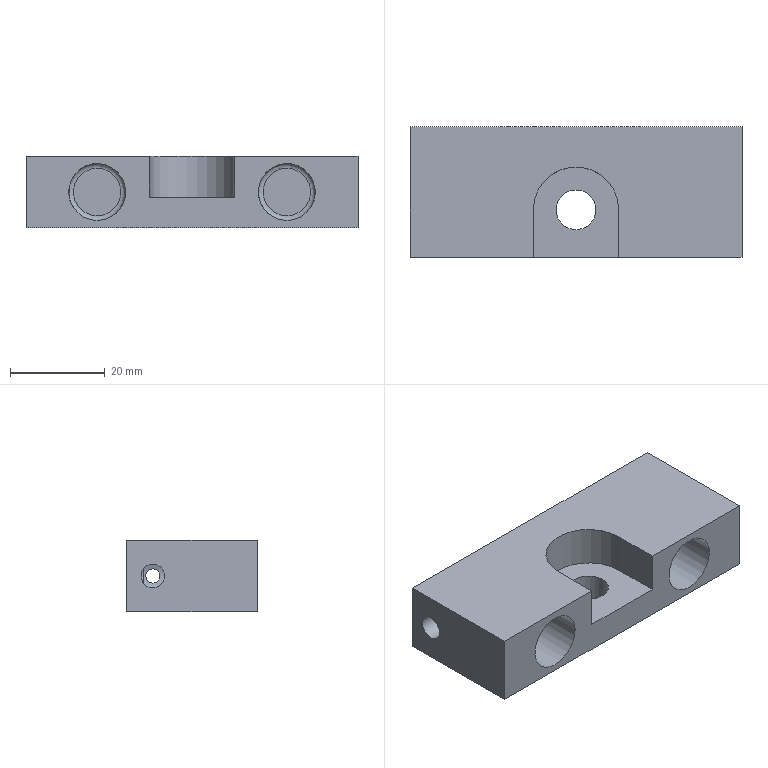NC program | NX | posted with a generic post | part box 70 x 27.5 x 15 mm
Lines 1 to 1563 of 3352, first 1339 of 1557 lines:
N10 G17 G21 G94 G90
(PLANAR_MILL_COPY , TOOL : D50面刀)
N12 T01 M6
N14 G53
N16 G17 G0 G90 X-0.05 Y-65. B0. C0. S1600 M3
N18 G43 Z20. H1
N20 Z3.05
N22 G94 G1 Z0.05 F800.
N24 Y-35.
N26 Y35.
N28 Y65.
N30 Z3.05
N32 G0 Z20.
N34 M5
(ADAPTIVE_MILLING , TOOL : D10-30-D10-75-3T-ROUGH)
N36 T02 M6
N38 G53
N40 G17 G0 G90 X-0.54 Y47.029 B0. C0. S3000 M3
N42 G43 Z20. H2
N44 Z-13.
N46 G94 G1 X-0.546 Y46.879 Z-13.937 F1500.
N48 X-0.553 Y46.729 Z-14.308
N50 X-0.559 Y46.579 Z-14.58
N52 X-0.566 Y46.43 Z-14.8
N54 X-0.572 Y46.28 Z-14.984
N56 X-0.579 Y46.13 Z-15.142
N58 X-0.586 Y45.98 Z-15.28
N60 X-0.592 Y45.83 Z-15.4
N62 X-0.599 Y45.68 Z-15.505
N64 X-0.605 Y45.53 Z-15.598
N66 X-0.612 Y45.381 Z-15.679
N68 X-0.618 Y45.231 Z-15.75
N70 X-0.625 Y45.081 Z-15.81
N72 X-0.631 Y44.931 Z-15.862
N74 X-0.638 Y44.781 Z-15.905
N76 X-0.644 Y44.631 Z-15.939
N78 X-0.651 Y44.481 Z-15.966
N80 X-0.657 Y44.332 Z-15.985
N82 X-0.664 Y44.182 Z-15.996
N84 X-0.67 Y44.032 Z-16.
N86 X-0.736 Y42.523
N88 G3 X0.007 Y41.505 R1.01
N90 X2.762 Y41.25 R14.191
N92 X13.643 Y41.189 R765.773
N94 G2 X17.871 Y38.648 R5.724
N96 X19.406 Y34.419 R9.683
N98 X19.682 Y29.331 R40.052
N100 G1 X19.699 Y22.431
N102 X19.698 Y-34.945
N104 G2 X17.285 Y-39.28 R5.638
N106 X12.977 Y-40.9 R9.483
N108 X7.401 Y-41.187 R42.459
N110 G1 X1.251 Y-41.2
N112 X-13.457 Y-41.198
N114 G2 X-17.775 Y-38.771 R5.666
N116 X-19.389 Y-34.525 R9.459
N118 X-19.681 Y-29.4 R38.334
N120 G1 X-19.699 Y-22.425
N122 X-19.697 Y34.946
N124 G2 X-17.282 Y39.268 R5.662
N126 X-13.075 Y40.881 R9.398
N128 X-7.988 Y41.181 R37.246
N130 X-1.014 Y41.164 R160.579
N132 G3 X9.001 Y40.903 R137.343
N134 G2 X12.406 Y40.86 R48.622
N136 X15.192 Y39.92 R6.998
N138 G1 X15.722 Y39.757
N140 G2 X17.393 Y38.64 R5.993
N142 X18.508 Y36.969 R5.993
N144 X19.081 Y34.188 R11.725
N146 X19.383 Y27.636 R61.147
N148 G1 X19.399 Y20.661
N150 X19.398 Y-33.278
N152 G2 X18.8 Y-36.008 R7.984
N154 X18.031 Y-37.862 R6.016
N156 X16.61 Y-39.283 R5.993
N158 X14.177 Y-40.223 R7.334
N160 X8.446 Y-40.842 R28.015
N162 X0.271 Y-40.899 R504.458
N164 G1 X-12.054 Y-40.887
N166 G2 X-15.177 Y-39.924 R6.927
N168 G1 X-15.722 Y-39.757
N170 G2 X-17.393 Y-38.64 R5.993
N172 X-18.508 Y-36.969 R5.993
N174 X-19.089 Y-34.118 R11.94
N176 X-19.388 Y-26.965 R67.131
N178 G1 X-19.399 Y-20.59
N180 X-19.398 Y33.255
N182 G2 X-18.803 Y35.985 R7.776
N184 X-18.031 Y37.862 R5.939
N186 X-16.61 Y39.283 R5.993
N188 X-14.212 Y40.213 R7.235
N190 X-8.557 Y40.838 R27.584
N192 X-3.607 Y40.895 R550.386
N194 X9.582 Y40.88 R989.035
N196 G3 X11.662 Y40.601 R75.414
N198 G2 X13.481 Y40.154 R43.193
N200 X15.722 Y39.757 R6.086
N202 X17.393 Y38.64 R5.993
N204 X18.508 Y36.969 R5.993
N206 X18.9 Y34.999 R5.998
N208 G3 X19.057 Y29. R461.095
N210 G2 X19.099 Y19.4 R690.026
N212 G1 X19.093 Y-32.197
N214 G2 X18.9 Y-33.872 R19.687
N216 X18.801 Y-36.006 R11.828
N218 G1 X18.735 Y-36.221
N220 G3 X20.129 Y-37.412 R1.
N222 X20.586 Y-36.97 Z-15.968 R1.088
N224 G1 X21.31 Y-35.839 Z-15.9
N226 X21.969 Y-34.809 F15000.
N228 G3 X22.127 Y-34.263 R1.011
N230 G1 X21.669 Y31.517
N232 X21.658 Y31.648
N234 X21.633 Y31.777
N236 X21.391 Y32.652
N238 X20.859 Y34.569 Z-16. F1500.
N240 G3 X18.9 Y34.287 R1.
N242 G1 Y-35.001
N244 G2 X18.507 Y-36.972 R5.996
N246 X17.39 Y-38.643 R5.993
N248 X15.719 Y-39.758 R5.993
N250 X13.749 Y-40.15 R5.998
N252 X4.104 Y-40.588 R90.538
N254 G1 X-2.421 Y-40.599
N256 G2 X-10.891 Y-40.577 R486.467
N258 X-13.286 Y-40.152 R14.802
N260 X-14.756 Y-40.051 R10.569
N262 G1 X-15.223 Y-39.909
N264 G3 X-16.353 Y-41.41 R1.
N266 X-15.967 Y-41.762 Z-15.974 R1.15
N268 G1 X-14.733 Y-42.546 Z-15.9
N270 X-13.791 Y-43.145 F15000.
N272 G3 X-13.264 Y-43.301 R1.013
N274 G1 X11.791 Y-43.542
N276 G3 X12.382 Y-43.356 R1.009
N278 G1 X13.375 Y-42.646
N280 X14.383 Y-41.921 Z-15.963 F1500.
N282 G3 X14.74 Y-41.285 Z-16. R1.001
N284 X13.749 Y-40.15 R1.
N286 X6.074 Y-40.264 R279.217
N288 G2 X-9.795 Y-40.283 R887.959
N290 G1 X-11.175 Y-40.15
N292 X-13.35
N294 G3 X-13.663 Y-42.1 R1.
N296 G1 X-11.746 Y-42.633 Z-15.9
N298 X-11.233 Y-42.78 F15000.
N300 X-10.716 Y-42.91
N302 X-10.581 Y-42.919
N304 X8.467
N306 X8.602 Y-42.908
N308 X8.735 Y-42.883
N310 X9.608 Y-42.64
N312 X11.525 Y-42.108 Z-16. F1500.
N314 G3 X11.237 Y-40.15 R1.
N316 G1 X-13.751
N318 G2 X-15.722 Y-39.757 R5.996
N320 X-17.393 Y-38.64 R5.993
N322 X-18.508 Y-36.969 R5.993
N324 X-18.9 Y-34.999 R5.998
N326 G3 X-19.058 Y-28.948 R473.561
N328 G2 X-19.099 Y-19.424 R689.078
N330 G1 X-19.097 Y31.83
N332 G2 X-18.9 Y33.843 R14.392
N334 X-18.801 Y36.006 R11.963
N336 G3 X-20.035 Y37.075 R1.
N338 X-20.677 Y36.588 Z-15.958 R1.059
N340 G1 X-21.331 Y35.628 Z-15.9
N342 X-22.019 Y34.619 F15000.
N344 G3 X-22.193 Y34.048 R1.009
N346 G1 X-21.669 Y-31.517
N348 X-21.658 Y-31.648
N350 X-21.633 Y-31.776
N352 X-21.391 Y-32.651
N354 X-20.859 Y-34.569 Z-16. F1500.
N356 G3 X-18.9 Y-34.287 R1.
N358 G1 Y35.001
N360 G2 X-18.507 Y36.972 R5.996
N362 X-17.39 Y38.643 R5.993
N364 X-15.719 Y39.758 R5.993
N366 X-13.75 Y40.15 R5.999
N368 X-3.9 Y40.588 R91.992
N370 G1 X1.425 Y40.595
N372 X8.533 Y40.593
N374 G2 X11.957 Y40.15 R25.662
N376 G1 X13.532
N378 G3 X14.526 Y41.262 R1.
N380 X14.033 Y42.02 Z-15.953 R1.045
N382 G1 X13.175 Y42.631 Z-15.9
N384 X12.153 Y43.357 F15000.
N386 G3 X11.574 Y43.542 R1.008
N388 G1 X-11.792
N390 G3 X-12.371 Y43.357 R1.008
N392 G1 X-13.372 Y42.646
N394 X-14.382 Y41.922 Z-15.963 F1500.
N396 G3 X-14.74 Y41.288 Z-16. R1.001
N398 X-13.75 Y40.15 R1.
N400 X-6.022 Y40.264 R288.131
N402 G2 X7.82 Y40.273 R666.629
N404 G1 X9.517 Y40.15
N406 X11.992
N408 G3 X12.305 Y42.1 R1.
N410 G1 X10.388 Y42.633 Z-15.9
N412 X9.875 Y42.78 F15000.
N414 X9.358 Y42.91
N416 X9.223 Y42.919
N418 X-8.506
N420 X-8.64 Y42.908
N422 X-8.773 Y42.883
N424 X-9.646 Y42.64
N426 X-11.563 Y42.108 Z-16. F1500.
N428 G3 X-11.275 Y40.15 R1.
N430 G1 X9.537
N432 G3 X10.535 Y41.321 R1.01
N434 G1 X10.322 Y42.637
N436 X10.298 Y42.785 Z-15.996
N438 X10.274 Y42.933 Z-15.985
N440 X10.25 Y43.081 Z-15.966
N442 X10.227 Y43.229 Z-15.939
N444 X10.203 Y43.377 Z-15.905
N446 X10.179 Y43.525 Z-15.862
N448 X10.155 Y43.673 Z-15.81
N450 X10.131 Y43.821 Z-15.75
N452 X10.107 Y43.969 Z-15.679
N454 X10.083 Y44.118 Z-15.598
N456 X10.059 Y44.266 Z-15.505
N458 X10.035 Y44.414 Z-15.4
N460 X10.011 Y44.562 Z-15.28
N462 X9.988 Y44.71 Z-15.142
N464 X9.964 Y44.858 Z-14.984
N466 X9.94 Y45.006 Z-14.8
N468 X9.916 Y45.154 Z-14.58
N470 X9.892 Y45.302 Z-14.308
N472 X9.868 Y45.45 Z-13.937
N474 X9.844 Y45.598 Z-13.
N476 G0 Z20.
N478 X-24.359 Y-10.135
N480 Z-5.499
N482 G1 X-24.21 Y-10.115 Z-6.436
N484 X-24.062 Y-10.095 Z-6.807
N486 X-23.913 Y-10.074 Z-7.079
N488 X-23.765 Y-10.054 Z-7.299
N490 X-23.616 Y-10.034 Z-7.483
N492 X-23.467 Y-10.014 Z-7.641
N494 X-23.319 Y-9.993 Z-7.779
N496 X-23.17 Y-9.973 Z-7.899
N498 X-23.021 Y-9.953 Z-8.004
N500 X-22.873 Y-9.932 Z-8.097
N502 X-22.724 Y-9.912 Z-8.178
N504 X-22.576 Y-9.892 Z-8.249
N506 X-22.427 Y-9.871 Z-8.309
N508 X-22.278 Y-9.851 Z-8.361
N510 X-22.13 Y-9.831 Z-8.404
N512 X-21.981 Y-9.81 Z-8.438
N514 X-21.833 Y-9.79 Z-8.465
N516 X-21.684 Y-9.77 Z-8.484
N518 X-21.535 Y-9.749 Z-8.495
N520 X-21.387 Y-9.729 Z-8.499
N522 X-19.729 Y-9.503
N524 G3 X-18.861 Y-8.601 R1.01
N526 X-18.61 Y-3.113 R44.979
N528 X-18.604 Y7.322 R791.192
N530 G2 X-18.864 Y8.631 R4.427
N532 G3 X-21.014 Y8.833 R1.1
N534 X-21.057 Y8.32 Z-8.473 R1.658
N536 G1 X-21.047 Y6.847 Z-8.399
N538 X-20.961 Y-6.535 F15000.
N540 X-20.948 Y-7.751 Z-8.46 F1500.
N542 G3 X-20.641 Y-8.442 Z-8.499 R1.101
N544 X-18.801 Y-7.994 R1.1
N546 X-18.4 Y-5.172 R11.11
N548 X-18.323 Y6.524 R244.406
N550 G1 X-18.411 Y6.848
N552 G3 X-19.933 Y7.308 R1.1
N554 X-20.494 Y6.285 Z-8.437 R1.133
N556 G1 X-20.515 Y5.523 Z-8.399
N558 X-20.832 Y-6.142 F15000.
N560 X-20.862 Y-7.434 Z-8.464 F1500.
N562 G3 X-20.624 Y-8.075 Z-8.499 R1.102
N564 X-18.713 Y-7.707 R1.1
N566 X-18.124 Y-4.24 R12.163
N568 X-18.029 Y5.649 R169.285
N570 X-18.164 Y6.386 R2.632
N572 G2 X-18.628 Y7.425 R3.79
N574 G3 X-20.442 Y7.9 R1.1
N576 X-20.779 Y6.991 Z-8.449 R1.147
N578 G1 X-20.764 Y6.004 Z-8.399
N580 X-20.59 Y-5.636 F15000.
N582 X-20.57 Y-6.604 Z-8.448 F1500.
N584 G3 X-20.058 Y-7.444 Z-8.499 R1.099
N586 X-18.507 Y-7.028 R1.1
N588 X-17.96 Y-4.778 R6.799
N590 X-17.713 Y1.504 R64.517
N592 X-17.785 Y5.427 R37.651
N594 X-17.984 Y6.075 R1.569
N596 X-19.388 Y6.427 R1.1
N598 X-19.99 Y5.405 Z-8.436 R1.127
N600 G1 X-20.024 Y4.667 Z-8.399
N602 X-20.481 Y-5.436 F15000.
N604 X-20.521 Y-6.436 Z-8.449 F1500.
N606 G3 X-20.089 Y-7.286 Z-8.499 R1.099
N608 X-18.454 Y-6.929 R1.1
N610 X-17.731 Y-4.48 R6.474
N612 X-17.422 Y1.708 R53.159
N614 X-17.541 Y5.13 R22.267
N616 X-18.033 Y6.14 R1.665
N618 G1 X-18.174 Y6.405
N620 G3 X-19.711 Y6.829 R1.1
N622 X-20.245 Y5.8 Z-8.438 R1.133
N624 G1 X-20.252 Y5.03 Z-8.399
N626 X-20.34 Y-5.168 F15000.
N628 X-20.342 Y-6.147 Z-8.448 F1500.
N630 G3 X-19.86 Y-6.993 Z-8.499 R1.099
N632 X-18.277 Y-6.598 R1.1
N634 X-17.479 Y-4.048 R6.758
N636 X-17.198 Y4.121 R47.526
N638 X-17.535 Y5.528 R3.358
N640 G1 X-17.818 Y5.878
N642 G3 X-19.188 Y6.149 R1.1
N644 X-19.77 Y5.122 Z-8.437 R1.128
N646 G1 X-19.794 Y4.377 Z-8.399
N648 X-20.088 Y-4.732 F15000.
N650 X-20.114 Y-5.693 Z-8.447 F1500.
N652 G3 X-19.635 Y-6.559 Z-8.499 R1.099
N654 X-18.047 Y-6.168 R1.1
N656 X-17.31 Y-4.123 R5.453
N658 X-16.865 Y1.668 R34.498
N660 X-17.096 Y4.751 R13.069
N662 X-17.379 Y5.348 R1.45
N664 X-18.583 Y5.473 R1.101
N666 X-19.18 Y4.487 Z-8.438 R1.134
N668 G1 X-19.241 Y3.711 Z-8.399
N670 X-19.887 Y-4.47 F15000.
N672 X-19.954 Y-5.405 Z-8.446 F1500.
N674 G3 X-19.496 Y-6.306 Z-8.499 R1.099
N676 X-18.007 Y-6.109 R1.1
N678 X-17.173 Y-4.263 R4.393
N680 X-16.612 Y0.923 R25.278
N682 X-16.83 Y4.394 R14.374
N684 X-17.249 Y5.242 R1.676
N686 X-18.475 Y5.353 R1.1
N688 X-19.048 Y4.387 Z-8.44 R1.131
N690 G1 X-19.113 Y3.577 Z-8.399
N692 X-19.743 Y-4.295 F15000.
N694 X-19.812 Y-5.23 Z-8.446 F1500.
N696 G3 X-19.355 Y-6.131 Z-8.499 R1.099
N698 X-17.865 Y-5.935 R1.1
N700 X-16.918 Y-3.908 R4.707
N702 X-16.461 Y3.485 R23.099
N704 X-16.927 Y4.948 R3.387
N706 X-17.393 Y5.36 R12.87
N708 G1 X-17.559 Y5.563
N710 G3 X-18.947 Y5.825 R1.1
N712 X-19.511 Y4.785 Z-8.436 R1.128
N714 G1 X-19.519 Y4.042 Z-8.399
N716 X-19.614 Y-4.137 F15000.
N718 X-19.619 Y-5.073 Z-8.446 F1500.
N720 G3 X-19.101 Y-5.942 Z-8.499 R1.099
N722 X-17.674 Y-5.703 R1.1
N724 X-16.676 Y-3.628 R4.873
N726 X-16.221 Y3.267 R19.842
N728 X-16.713 Y4.773 R3.545
N730 G1 X-17.055 Y5.083
N732 G3 X-18.304 Y5.185 R1.1
N734 X-18.857 Y4.21 Z-8.44 R1.131
N736 G1 X-18.907 Y3.396 Z-8.399
N738 X-19.355 Y-3.822 F15000.
N740 X-19.407 Y-4.757 Z-8.446 F1500.
N742 G3 X-18.933 Y-5.651 Z-8.499 R1.099
N744 X-17.46 Y-5.442 R1.1
N746 X-16.448 Y-3.413 R4.805
N748 X-15.99 Y3.086 R17.275
N750 X-16.502 Y4.606 R3.475
N752 G1 X-16.605 Y4.714
N754 G3 X-17.695 Y4.721 R1.101
N756 X-18.259 Y3.791 Z-8.442 R1.135
N758 G1 X-18.355 Y2.943 Z-8.399
N760 X-19.085 Y-3.532 F15000.
N762 X-19.184 Y-4.464 Z-8.446 F1500.
N764 G3 X-18.757 Y-5.38 Z-8.499 R1.099
N766 X-17.39 Y-5.357 R1.1
N768 X-16.443 Y-3.867 R3.519
N770 X-15.796 Y3.107 R14.715
N772 X-16.339 Y4.508 R3.093
N774 G1 X-16.508 Y4.656
N776 G3 X-17.672 Y4.687 R1.076
N778 X-18.193 Y3.791 Z-8.445 R1.108
N780 G1 X-18.289 Y2.887 Z-8.399
N782 X-18.956 Y-3.418 F15000.
N784 X-19.057 Y-4.417 Z-8.45 F1500.
N786 G3 X-18.669 Y-5.284 Z-8.499 R1.074
N788 X-17.303 Y-5.286 R1.075
N790 X-16.245 Y-3.739 R3.537
N792 X-15.582 Y2.989 R13.284
N794 X-16.211 Y4.462 R2.96
N796 G1 X-16.389 Y4.6
N798 G3 X-17.497 Y4.558 R1.101
N800 X-18.011 Y3.665 Z-8.445 R1.135
N802 G1 X-18.116 Y2.752 Z-8.399
N804 X-18.82 Y-3.305 F15000.
N806 X-18.923 Y-4.246 Z-8.447 F1500.
N808 G3 X-18.506 Y-5.158 Z-8.499 R1.099
N810 X-17.13 Y-5.143 R1.1
N812 X-15.966 Y-3.424 R3.809
N814 X-15.372 Y2.873 R12.173
N816 X-16.029 Y4.366 R3.073
N818 X-16.612 Y4.719 R3.315
N820 G1 X-16.844 Y4.909
N822 G3 X-18.123 Y4.993 R1.1
N824 X-18.643 Y3.972 Z-8.439 R1.135
N826 G1 X-18.651 Y3.186 Z-8.399
N828 X-18.715 Y-3.217 F15000.
N830 X-18.719 Y-4.193 Z-8.448 F1500.
N832 G3 X-18.235 Y-5.041 Z-8.499 R1.099
N834 X-16.927 Y-4.977 R1.1
N836 X-15.766 Y-3.309 R3.83
N838 X-15.188 Y2.856 R11.082
N840 X-15.852 Y4.278 R2.951
N842 G1 X-16.213 Y4.505
N844 G3 X-17.353 Y4.443 R1.101
N846 X-17.836 Y3.543 Z-8.446 R1.141
N848 G1 X-17.921 Y2.618 Z-8.399
N850 X-18.437 Y-2.99 F15000.
N852 X-18.518 Y-3.939 Z-8.447 F1500.
N854 G3 X-18.084 Y-4.838 Z-8.499 R1.099
N856 X-16.724 Y-4.81 R1.1
N858 X-15.513 Y-3.07 R3.925
N860 X-14.989 Y2.763 R10.298
N862 X-15.669 Y4.184 R2.932
N864 G1 X-16.019 Y4.401
N866 G3 X-17.169 Y4.332 R1.101
N868 X-17.641 Y3.429 Z-8.446 R1.141
N870 G1 X-17.718 Y2.5 Z-8.399
N872 X-18.151 Y-2.758 F15000.
N874 X-18.225 Y-3.734 Z-8.448 F1500.
N876 G3 X-17.806 Y-4.613 Z-8.499 R1.099
N878 X-16.61 Y-4.717 R1.101
N880 X-15.502 Y-3.375 R3.126
N882 X-14.824 Y2.793 R9.464
N884 X-15.501 Y4.105 R2.672
N886 G1 X-15.689 Y4.229
N888 G3 X-16.713 Y4.111 R1.101
N890 X-17.192 Y3.261 Z-8.448 R1.146
N892 G1 X-17.329 Y2.29 Z-8.399
N894 X-18.026 Y-2.669 F15000.
N896 X-18.157 Y-3.636 Z-8.448 F1500.
N898 G3 X-17.786 Y-4.54 Z-8.499 R1.099
N900 X-16.544 Y-4.682 R1.1
N902 X-15.34 Y-3.336 R3.03
N904 X-14.661 Y2.809 R8.843
N906 X-15.389 Y4.082 R2.488
N908 G1 X-15.584 Y4.194
N910 G3 X-16.642 Y4.071 R1.076
N912 X-17.083 Y3.254 Z-8.451 R1.12
N914 G1 X-17.219 Y2.231 Z-8.399
N916 X-17.856 Y-2.561 F15000.
N918 X-17.988 Y-3.594 Z-8.451 F1500.
N920 G3 X-17.653 Y-4.447 Z-8.499 R1.075
N922 X-16.411 Y-4.611 R1.075
N924 X-15.16 Y-3.267 R3.047
N926 X-14.482 Y2.764 R8.386
N928 X-15.255 Y4.05 R2.497
N930 G1 X-15.487 Y4.171
N932 G3 X-16.479 Y3.989 R1.101
N934 X-16.909 Y3.181 Z-8.452 R1.147
N936 G1 X-17.058 Y2.144 Z-8.399
N938 X-17.722 Y-2.486 F15000.
N940 X-17.859 Y-3.472 Z-8.449 F1500.
N942 G3 X-17.507 Y-4.364 Z-8.499 R1.099
N944 X-16.246 Y-4.523 R1.1
N946 X-14.951 Y-3.148 R3.109
N948 X-14.321 Y2.761 R7.947
N950 X-15.123 Y4.021 R2.428
N952 X-15.722 Y4.243 R2.988
N954 G1 X-15.821 Y4.296
N956 G3 X-16.992 Y4.212 R1.101
N958 X-17.443 Y3.272 Z-8.445 R1.134
N960 G1 X-17.473 Y2.367 Z-8.399
N962 X-17.633 Y-2.437 F15000.
N964 X-17.655 Y-2.996 Z-8.427 F1500.
N966 X-17.66 Y-3.555 Z-8.455
N968 G3 X-17.258 Y-4.301 Z-8.499 R1.116
N970 X-16.048 Y-4.417 R1.101
N972 X-14.743 Y-3.032 R3.144
N974 X-14.136 Y2.681 R7.63
N976 X-14.939 Y3.959 R2.556
N978 X-15.352 Y4.13 R2.709
N980 X-16.379 Y3.92 R1.101
N982 X-16.776 Y3.101 Z-8.452 R1.148
N984 G1 X-16.889 Y2.054 Z-8.399
N986 X-17.36 Y-2.292 F15000.
N988 X-17.464 Y-3.297 Z-8.45 F1500.
N990 G3 X-17.093 Y-4.167 Z-8.499 R1.099
N992 X-15.849 Y-4.311 R1.1
N994 X-14.497 Y-2.846 R3.242
N996 X-13.955 Y2.608 R7.351
N998 X-14.786 Y3.919 R2.545
N1000 X-15.205 Y4.086 R3.378
N1002 X-16.259 Y3.853 R1.101
N1004 X-16.629 Y3.027 Z-8.452 R1.149
N1006 G1 X-16.716 Y1.973 Z-8.399
N1008 X-17.051 Y-2.127 F15000.
N1010 X-17.101 Y-2.684 Z-8.427 F1500.
N1012 X-17.133 Y-3.243 Z-8.455
N1014 G3 X-16.768 Y-4.008 Z-8.499 R1.116
N1016 X-15.719 Y-4.242 R1.101
N1018 X-14.47 Y-3.047 R2.783
N1020 X-13.824 Y2.677 R6.992
N1022 X-14.655 Y3.889 R2.357
N1024 G1 X-15.004 Y4.025
N1026 G3 X-16.061 Y3.788 R1.101
N1028 X-16.427 Y3.007 Z-8.455 R1.156
N1030 G1 X-16.554 Y1.909 Z-8.399
N1032 X-17.021 Y-2.111 F15000.
N1034 X-17.135 Y-3.136 Z-8.451 F1500.
N1036 G3 X-16.787 Y-3.995 Z-8.499 R1.1
N1038 X-15.719 Y-4.242 R1.101
N1040 X-14.423 Y-3.181 R2.503
N1042 X-13.661 Y2.65 R6.743
N1044 X-14.495 Y3.844 R2.327
N1046 G1 X-14.735 Y3.947
N1048 G3 X-15.624 Y3.661 R1.102
N1050 X-15.976 Y2.944 Z-8.458 R1.166
N1052 G1 X-16.172 Y1.787 Z-8.399
N1054 X-16.817 Y-2.007 F15000.
N1056 X-16.914 Y-2.555 Z-8.427 F1500.
N1058 X-16.994 Y-3.106 Z-8.455
N1060 G3 X-16.692 Y-3.904 Z-8.499 R1.116
N1062 X-15.576 Y-4.198 R1.101
N1064 X-14.281 Y-3.171 R2.53
N1066 X-13.506 Y2.644 R6.533
N1068 X-14.39 Y3.839 R2.261
N1070 G1 X-14.672 Y3.938
N1072 G3 X-15.612 Y3.656 R1.101
N1074 X-15.961 Y2.922 Z-8.457 R1.163
N1076 G1 X-16.133 Y1.776 Z-8.399
N1078 X-16.691 Y-1.947 F15000.
N1080 X-16.779 Y-2.512 Z-8.428 F1500.
N1082 X-16.851 Y-3.079 Z-8.457
N1084 G3 X-16.558 Y-3.85 Z-8.499 R1.116
N1086 X-15.432 Y-4.155 R1.101
N1088 X-14.034 Y-3.015 R2.664
N1090 X-13.354 Y2.637 R6.36
N1092 X-14.286 Y3.841 R2.249
N1094 G1 X-14.571 Y3.931
N1096 G3 X-15.474 Y3.618 R1.102
N1098 X-15.8 Y2.908 Z-8.459 R1.169
N1100 G1 X-15.982 Y1.73 Z-8.399
N1102 X-16.541 Y-1.891 F15000.
N1104 X-16.632 Y-2.459 Z-8.428 F1500.
N1106 X-16.707 Y-3.03 Z-8.457
N1108 G3 X-16.423 Y-3.797 Z-8.499 R1.116
N1110 X-15.289 Y-4.111 R1.101
N1112 X-13.932 Y-3.065 R2.58
N1114 X-13.237 Y2.709 R6.146
N1116 X-14.198 Y3.849 R2.143
N1118 G1 X-14.45 Y3.919
N1120 G3 X-15.352 Y3.583 R1.102
N1122 X-15.657 Y2.894 Z-8.46 R1.167
N1124 G1 X-15.838 Y1.686 Z-8.399
N1126 X-16.365 Y-1.833 F15000.
N1128 X-16.448 Y-2.376 Z-8.427 F1500.
N1130 X-16.522 Y-2.922 Z-8.454
N1132 G3 X-16.246 Y-3.74 Z-8.499 R1.1
N1134 X-15.109 Y-4.057 R1.101
N1136 X-13.748 Y-3. R2.604
N1138 X-13.048 Y2.612 R6.046
N1140 X-14.008 Y3.815 R2.338
N1142 X-14.756 Y3.949 R2.163
N1144 G1 X-14.828 Y3.971
N1146 G3 X-15.908 Y3.713 R1.101
N1148 X-16.249 Y2.844 Z-8.451 R1.145
N1150 G1 X-16.267 Y1.817 Z-8.399
N1152 X-16.33 Y-1.82 F15000.
N1154 X-16.345 Y-3.004 Z-8.459 F1500.
N1156 G3 X-16.03 Y-3.724 Z-8.499 R1.101
N1158 X-14.93 Y-4.002 R1.101
N1160 X-13.518 Y-2.871 R2.703
N1162 X-12.893 Y2.593 R5.932
N1164 X-13.881 Y3.808 R2.347
N1166 X-14.318 Y3.906 R2.088
N1168 X-15.244 Y3.547 R1.101
N1170 X-15.529 Y2.848 Z-8.46 R1.167
N1172 G1 X-15.673 Y1.636 Z-8.399
N1174 X-16.075 Y-1.744 F15000.
N1176 X-16.201 Y-2.855 Z-8.455 F1500.
N1178 G3 X-15.914 Y-3.652 Z-8.499 R1.1
N1180 X-14.786 Y-3.959 R1.101
N1182 X-13.383 Y-2.874 R2.623
N1184 X-12.784 Y2.674 R5.779
N1186 X-13.779 Y3.812 R2.199
N1188 X-14.203 Y3.895 R3.262
N1190 X-15.148 Y3.514 R1.101
N1192 X-15.415 Y2.813 Z-8.461 R1.168
N1194 G1 X-15.534 Y1.594 Z-8.399
N1196 X-15.852 Y-1.676 F15000.
N1198 X-15.958 Y-2.824 Z-8.457 F1500.
N1200 G3 X-15.678 Y-3.59 Z-8.499 R1.1
N1202 X-14.753 Y-3.949 R1.101
N1204 X-13.404 Y-3.074 R2.272
N1206 X-12.633 Y2.66 R5.667
N1208 X-13.608 Y3.788 R2.263
N1210 X-14.047 Y3.879 R2.429
N1212 X-15.006 Y3.482 R1.101
N1214 X-15.259 Y2.817 Z-8.463 R1.186
N1216 G1 X-15.408 Y1.559 Z-8.399
N1218 X-15.79 Y-1.658 F15000.
N1220 X-15.92 Y-2.797 Z-8.457 F1500.
N1222 G3 X-15.653 Y-3.574 Z-8.499 R1.1
N1224 X-14.716 Y-3.945 R1.101
N1226 X-13.364 Y-3.178 R2.142
N1228 X-12.529 Y2.743 R5.535
N1230 X-13.503 Y3.791 R2.11
N1232 G1 X-13.72 Y3.848
N1234 G3 X-14.661 Y3.418 R1.101
N1236 X-14.889 Y2.827 Z-8.467 R1.199
N1238 G1 X-15.1 Y1.495 Z-8.399
N1240 X-15.592 Y-1.599 F15000.
N1242 X-15.767 Y-2.739 Z-8.457 F1500.
N1244 G3 X-15.536 Y-3.52 Z-8.499 R1.1
N1246 X-14.567 Y-3.93 R1.101
N1248 X-13.136 Y-3.076 R2.291
N1250 X-12.38 Y2.732 R5.48
N1252 X-13.384 Y3.79 R2.106
N1254 G1 X-13.677 Y3.85
N1256 G3 X-14.559 Y3.404 R1.101
N1258 X-14.776 Y2.827 Z-8.468 R1.204
N1260 G1 X-14.991 Y1.479 Z-8.399
N1262 X-15.476 Y-1.564 F15000.
N1264 X-15.655 Y-2.725 Z-8.458 F1500.
N1266 G3 X-15.438 Y-3.49 Z-8.499 R1.101
N1268 X-14.455 Y-3.919 R1.101
N1270 X-13.09 Y-3.171 R2.202
N1272 X-12.232 Y2.723 R5.4
N1274 X-13.267 Y3.796 R2.115
N1276 X-13.863 Y3.861 R2.988
N1278 X-14.839 Y3.441 R1.101
N1280 X-15.075 Y2.757 Z-8.462 R1.183
N1282 G1 X-15.174 Y1.508 Z-8.399
N1284 X-15.416 Y-1.547 F15000.
N1286 X-15.469 Y-2.175 Z-8.431 F1500.
N1288 X-15.51 Y-2.804 Z-8.462
N1290 G3 X-15.284 Y-3.482 Z-8.499 R1.101
N1292 X-14.305 Y-3.905 R1.101
N1294 X-12.88 Y-3.095 R2.306
N1296 X-12.113 Y2.769 R5.347
N1298 X-13.153 Y3.801 R2.088
N1300 X-13.563 Y3.85 R2.846
N1302 X-14.452 Y3.397 R1.101
N1304 X-14.666 Y2.8 Z-8.467 R1.198
N1306 G1 X-14.844 Y1.465 Z-8.399
N1308 X-15.239 Y-1.505 F15000.
N1310 X-15.396 Y-2.723 Z-8.461 F1500.
N1312 G3 X-15.195 Y-3.44 Z-8.499 R1.102
N1314 X-14.193 Y-3.894 R1.101
N1316 X-12.727 Y-3.078 R2.302
N1318 X-11.966 Y2.761 R5.301
N1320 X-13.01 Y3.799 R2.138
N1322 X-13.435 Y3.85 R2.424
N1324 X-14.331 Y3.387 R1.101
N1326 X-14.538 Y2.795 Z-8.467 R1.201
N1328 G1 X-14.712 Y1.452 Z-8.399
N1330 X-15.092 Y-1.483 F15000.
N1332 X-15.247 Y-2.711 Z-8.461 F1500.
N1334 G3 X-15.05 Y-3.42 Z-8.499 R1.102
N1336 X-14.044 Y-3.879 R1.101
N1338 X-12.575 Y-3.063 R2.313
N1340 X-11.819 Y2.754 R5.263
N1342 X-12.881 Y3.802 R2.143
N1344 X-13.288 Y3.85 R2.966
N1346 X-14.193 Y3.375 R1.101
N1348 X-14.392 Y2.794 Z-8.468 R1.205
N1350 G1 X-14.567 Y1.437 Z-8.399
N1352 X-14.943 Y-1.463 F15000.
N1354 X-15.031 Y-2.113 Z-8.432 F1500.
N1356 X-15.103 Y-2.764 Z-8.465
N1358 G3 X-14.903 Y-3.401 Z-8.499 R1.129
N1360 X-13.895 Y-3.864 R1.101
N1362 X-12.348 Y-2.967 R2.398
N1364 X-11.683 Y2.766 R5.23
N1366 X-12.77 Y3.81 R2.108
N1368 X-13.158 Y3.85 R5.359
N1370 X-14.07 Y3.365 R1.101
N1372 X-14.262 Y2.771 Z-8.467 R1.201
N1374 G1 X-14.407 Y1.422 Z-8.399
N1376 X-14.715 Y-1.441 F15000.
N1378 X-14.785 Y-2.075 Z-8.431 F1500.
N1380 X-14.846 Y-2.711 Z-8.463
N1382 G3 X-14.65 Y-3.382 Z-8.499 R1.101
N1384 X-13.749 Y-3.85 R1.101
N1386 X-12.33 Y-3.097 R2.244
N1388 X-11.58 Y2.834 R5.161
N1390 X-12.633 Y3.812 R2.038
N1392 X-13.044 Y3.85 R4.431
N1394 X-13.962 Y3.356 R1.101
N1396 X-14.148 Y2.785 Z-8.469 R1.21
N1398 G1 X-14.314 Y1.413 Z-8.399
N1400 X-14.66 Y-1.435 F15000.
N1402 X-14.739 Y-2.066 Z-8.431 F1500.
N1404 X-14.808 Y-2.697 Z-8.463
N1406 G3 X-14.616 Y-3.376 Z-8.499 R1.101
N1408 X-13.712 Y-3.85 R1.101
N1410 X-12.299 Y-3.2 R2.093
N1412 X-10.895 Y1.296 R5.123
N1414 X-12.028 Y3.55 R3.752
N1416 X-12.882 Y3.85 R1.151
N1418 X-13.809 Y3.342 R1.101
N1420 X-13.997 Y2.705 Z-8.465 R1.413
N1422 G1 X-14.168 Y1.398 Z-8.399
N1424 X-14.536 Y-1.423 F15000.
N1426 X-14.62 Y-2.055 Z-8.431 F1500.
N1428 X-14.695 Y-2.687 Z-8.463
N1430 G3 X-14.511 Y-3.365 Z-8.499 R1.101
N1432 X-13.599 Y-3.85 R1.101
N1434 X-12.105 Y-3.15 R2.164
N1436 X-11.305 Y2.855 R5.101
N1438 X-12.356 Y3.813 R2.029
N1440 X-12.765 Y3.85 R4.963
N1442 X-13.698 Y3.333 R1.101
N1444 X-13.88 Y2.698 Z-8.466 R1.419
N1446 G1 X-14.043 Y1.386 Z-8.399
N1448 X-14.391 Y-1.409 F15000.
N1450 X-14.545 Y-2.692 Z-8.464 F1500.
N1452 G3 X-14.369 Y-3.353 Z-8.499 R1.102
N1454 X-13.449 Y-3.85 R1.101
N1456 X-11.975 Y-3.16 R2.198
N1458 X-11.206 Y2.926 R5.062
N1460 X-12.267 Y3.826 R1.916
N1462 G1 X-12.601 Y3.85
N1464 G3 X-13.541 Y3.323 R1.101
N1466 X-13.717 Y2.706 Z-8.466 R1.443
N1468 G1 X-13.895 Y1.376 Z-8.399
N1470 X-14.266 Y-1.397 F15000.
N1472 X-14.432 Y-2.681 Z-8.464 F1500.
N1474 G3 X-14.264 Y-3.342 Z-8.499 R1.102
N1476 X-13.337 Y-3.85 R1.101
N1478 X-11.799 Y-3.127 R2.216
N1480 X-11.034 Y2.882 R5.064
N1482 X-12.095 Y3.819 R1.983
N1484 G1 X-12.485 Y3.85
N1486 G3 X-13.427 Y3.318 R1.101
N1488 X-13.6 Y2.699 Z-8.466 R1.441
N1490 G1 X-13.77 Y1.37 Z-8.399
N1492 X-14.121 Y-1.382 F15000.
N1494 X-14.282 Y-2.686 Z-8.465 F1500.
N1496 G3 X-14.121 Y-3.33 Z-8.499 R1.103
N1498 X-13.187 Y-3.85 R1.101
N1500 X-11.669 Y-3.139 R2.224
N1502 X-10.889 Y2.88 R5.053
N1504 X-11.946 Y3.818 R2.002
N1506 G1 X-12.305 Y3.85
N1508 G3 X-13.249 Y3.315 R1.101
N1510 X-13.421 Y2.711 Z-8.467 R1.465
N1512 G1 X-13.609 Y1.369 Z-8.399
N1514 X-13.992 Y-1.37 F15000.
N1516 X-14.169 Y-2.672 Z-8.465 F1500.
N1518 G3 X-14.016 Y-3.318 Z-8.499 R1.103
N1520 X-13.074 Y-3.85 R1.101
N1522 X-11.551 Y-3.163 R2.213
N1524 X-10.778 Y2.932 R5.025
N1526 X-11.82 Y3.822 R1.931
N1528 G1 X-12.156 Y3.85
N1530 G3 X-13.099 Y3.315 R1.101
N1532 X-13.272 Y2.711 Z-8.467 R1.465
N1534 G1 X-13.459 Y1.368 Z-8.399
N1536 X-13.841 Y-1.362 F15000.
N1538 X-14.019 Y-2.672 Z-8.465 F1500.
N1540 G3 X-13.87 Y-3.312 Z-8.499 R1.103
N1542 X-12.924 Y-3.85 R1.101
N1544 X-11.421 Y-3.175 R2.21
N1546 X-10.606 Y2.89 R5.026
N1548 X-11.659 Y3.818 R1.996
N1550 G1 X-12.023 Y3.85
N1552 G3 X-12.967 Y3.316 R1.101
N1554 X-13.139 Y2.708 Z-8.467 R1.459
N1556 G1 X-13.322 Y1.368 Z-8.399
N1558 X-13.694 Y-1.358 F15000.
N1560 X-13.869 Y-2.674 Z-8.466 F1500.
N1562 G3 X-13.722 Y-3.308 Z-8.499 R1.103
N1564 X-12.774 Y-3.85 R1.101
N1566 X-11.237 Y-3.138 R2.247
N1568 X-10.494 Y2.941 R5.015
N1570 X-11.539 Y3.824 R1.923
N1572 G1 X-11.874 Y3.85
N1574 G3 X-12.818 Y3.316 R1.101
N1576 X-12.99 Y2.707 Z-8.467 R1.459
N1578 G1 X-13.173 Y1.368 Z-8.399
N1580 X-13.545 Y-1.358 F15000.
N1582 X-13.719 Y-2.675 Z-8.466 F1500.
N1584 G3 X-13.572 Y-3.308 Z-8.499 R1.103
N1586 X-12.624 Y-3.85 R1.101
N1588 X-11.109 Y-3.153 R2.265
N1590 X-10.336 Y2.919 R5.013
N1592 X-11.383 Y3.821 R1.958
N1594 G1 X-11.761 Y3.85
N1596 G3 X-12.704 Y3.316 R1.101
N1598 X-12.877 Y2.708 Z-8.467 R1.459
N1600 G1 X-13.06 Y1.368 Z-8.399
N1602 X-13.432 Y-1.358 F15000.
N1604 X-13.607 Y-2.674 Z-8.466 F1500.
N1606 G3 X-13.46 Y-3.308 Z-8.499 R1.103
N1608 X-12.512 Y-3.85 R1.101
N1610 X-10.961 Y-3.149 R2.245
N1612 X-10.191 Y2.918 R5.007
N1614 X-11.236 Y3.82 R1.965
N1616 G1 X-11.584 Y3.85
N1618 G3 X-12.528 Y3.314 R1.101
N1620 X-12.7 Y2.712 Z-8.467 R1.469
N1622 G1 X-12.89 Y1.368 Z-8.399
N1624 X-13.276 Y-1.358 F15000.
N1626 X-13.456 Y-2.67 Z-8.466 F1500.
N1628 G3 X-13.31 Y-3.307 Z-8.499 R1.103
N1630 X-12.362 Y-3.85 R1.101
N1632 X-10.824 Y-3.156 R2.246
N1634 X-10.044 Y2.914 R5.004
N1636 X-11.105 Y3.823 R1.948
N1638 G1 X-11.44 Y3.85
N1640 G3 X-12.384 Y3.315 R1.101
N1642 X-12.557 Y2.711 Z-8.467 R1.466
N1644 G1 X-12.745 Y1.368 Z-8.399
N1646 X-13.127 Y-1.358 F15000.
N1648 X-13.306 Y-2.671 Z-8.466 F1500.
N1650 G3 X-13.16 Y-3.308 Z-8.499 R1.103
N1652 X-12.212 Y-3.85 R1.101
N1654 X-10.684 Y-3.161 R2.246
N1656 X-9.885 Y2.893 R5.002
N1658 X-10.933 Y3.817 R2.004
N1660 G1 X-11.301 Y3.85
N1662 G3 X-12.245 Y3.315 R1.101
N1664 X-12.417 Y2.709 Z-8.467 R1.463
N1666 G1 X-12.603 Y1.368 Z-8.399
N1668 X-12.98 Y-1.358 F15000.
N1670 X-13.157 Y-2.673 Z-8.466 F1500.
N1672 G3 X-13.01 Y-3.308 Z-8.499 R1.103
N1674 X-12.062 Y-3.85 R1.101
N1676 X-10.547 Y-3.169 R2.24
N1678 X-9.751 Y2.91 R4.997
N1680 X-10.813 Y3.823 R1.956
N1682 G1 X-11.186 Y3.85
N1684 G3 X-12.129 Y3.316 R1.101
N1686 X-12.302 Y2.703 Z-8.467 R1.451
N1688 G1 X-12.478 Y1.368 Z-8.399
N1690 X-12.838 Y-1.358 F15000.
N1692 X-13.007 Y-2.679 Z-8.466 F1500.
N1694 G3 X-12.859 Y-3.309 Z-8.499 R1.103
N1696 X-11.912 Y-3.85 R1.101
N1698 X-10.387 Y-3.155 R2.256
N1700 X-9.59 Y2.885 R5.004
N1702 X-10.647 Y3.818 R2.009
N1704 G1 X-11.011 Y3.85
N1706 G3 X-11.955 Y3.315 R1.101
N1708 X-12.127 Y2.707 Z-8.467 R1.459
N1710 G1 X-12.31 Y1.368 Z-8.399
N1712 X-12.682 Y-1.358 F15000.
N1714 X-12.857 Y-2.674 Z-8.466 F1500.
N1716 G3 X-12.71 Y-3.308 Z-8.499 R1.103
N1718 X-11.762 Y-3.85 R1.101
N1720 X-10.161 Y-3.079 R2.34
N1722 X-9.455 Y2.9 R5.014
N1724 X-10.519 Y3.822 R1.978
N1726 G1 X-10.892 Y3.85
N1728 G3 X-11.836 Y3.315 R1.101
N1730 X-12.008 Y2.709 Z-8.467 R1.462
N1732 G1 X-12.192 Y1.368 Z-8.399
N1734 X-12.568 Y-1.358 F15000.
N1736 X-12.744 Y-2.673 Z-8.466 F1500.
N1738 G3 X-12.597 Y-3.308 Z-8.499 R1.103
N1740 X-11.649 Y-3.85 R1.101
N1742 X-10.132 Y-3.187 R2.231
N1744 X-9.321 Y2.918 R4.986
N1746 X-10.39 Y3.825 R1.95
N1748 G1 X-10.726 Y3.85
N1750 G3 X-11.67 Y3.314 R1.101
N1752 X-11.842 Y2.711 Z-8.467 R1.468
N1754 G1 X-12.031 Y1.368 Z-8.399
N1756 X-12.414 Y-1.358 F15000.
N1758 X-12.594 Y-2.67 Z-8.466 F1500.
N1760 G3 X-12.448 Y-3.307 Z-8.499 R1.103
N1762 X-11.499 Y-3.85 R1.101
N1764 X-9.949 Y-3.153 R2.26
N1766 X-9.187 Y2.934 R4.992
N1768 X-10.259 Y3.828 R1.908
N1770 G1 X-10.611 Y3.85
N1772 G3 X-11.555 Y3.315 R1.101
N1774 X-11.727 Y2.705 Z-8.467 R1.455
N1776 G1 X-11.907 Y1.368 Z-8.399
N1778 X-12.272 Y-1.358 F15000.
N1780 X-12.444 Y-2.677 Z-8.466 F1500.
N1782 G3 X-12.297 Y-3.308 Z-8.499 R1.103
N1784 X-11.349 Y-3.85 R1.101
N1786 X-9.797 Y-3.146 R2.262
N1788 X-9.051 Y2.948 R4.989
N1790 X-10.097 Y3.824 R1.929
N1792 G1 X-10.433 Y3.85
N1794 G3 X-11.377 Y3.314 R1.101
N1796 X-11.549 Y2.71 Z-8.467 R1.466
N1798 G1 X-11.736 Y1.368 Z-8.399
N1800 X-12.116 Y-1.358 F15000.
N1802 X-12.294 Y-2.672 Z-8.466 F1500.
N1804 G3 X-12.147 Y-3.308 Z-8.499 R1.103
N1806 X-11.199 Y-3.85 R1.101
N1808 X-9.66 Y-3.154 R2.259
N1810 X-8.881 Y2.909 R4.995
N1812 X-9.944 Y3.822 R1.968
N1814 G1 X-10.317 Y3.85
N1816 G3 X-11.26 Y3.315 R1.101
N1818 X-11.433 Y2.704 Z-8.467 R1.454
N1820 G1 X-11.611 Y1.368 Z-8.399
N1822 X-11.974 Y-1.358 F15000.
N1824 X-12.144 Y-2.678 Z-8.466 F1500.
N1826 G3 X-11.997 Y-3.308 Z-8.499 R1.103
N1828 X-11.049 Y-3.85 R1.101
N1830 X-9.521 Y-3.16 R2.252
N1832 X-8.784 Y2.982 R4.976
N1834 X-9.814 Y3.827 R1.877
N1836 G1 X-10.14 Y3.85
N1838 G3 X-11.084 Y3.314 R1.101
N1840 X-11.256 Y2.709 Z-8.467 R1.463
N1842 G1 X-11.441 Y1.367 Z-8.399
N1844 X-11.818 Y-1.358 F15000.
N1846 X-11.994 Y-2.673 Z-8.466 F1500.
N1848 G3 X-11.847 Y-3.308 Z-8.499 R1.103
N1850 X-10.899 Y-3.85 R1.101
N1852 X-9.37 Y-3.154 R2.261
N1854 X-8.628 Y2.965 R4.979
N1856 X-9.646 Y3.822 R1.919
N1858 G1 X-10.02 Y3.85
N1860 G3 X-10.963 Y3.315 R1.101
N1862 X-11.135 Y2.704 Z-8.467 R1.453
N1864 G1 X-11.313 Y1.367 Z-8.399
N1866 X-11.674 Y-1.358 F15000.
N1868 X-11.844 Y-2.678 Z-8.466 F1500.
N1870 G3 X-11.697 Y-3.309 Z-8.499 R1.103
N1872 X-10.749 Y-3.85 R1.101
N1874 X-9.239 Y-3.168 R2.25
N1876 X-8.439 Y2.898 R4.992
N1878 X-9.482 Y3.816 R2.011
N1880 G1 X-9.854 Y3.85
N1882 G3 X-10.799 Y3.313 R1.101
N1884 X-10.97 Y2.713 Z-8.467 R1.472
N1886 G1 X-11.162 Y1.367 Z-8.399
N1888 X-11.55 Y-1.358 F15000.
N1890 X-11.731 Y-2.669 Z-8.466 F1500.
N1892 G3 X-11.585 Y-3.307 Z-8.499 R1.103
N1894 X-10.637 Y-3.85 R1.101
N1896 X-9.108 Y-3.181 R2.24
N1898 X-8.295 Y2.899 R4.987
N1900 X-9.358 Y3.822 R1.982
N1902 G1 X-9.731 Y3.85
N1904 G3 X-10.675 Y3.314 R1.101
N1906 X-10.847 Y2.708 Z-8.467 R1.462
N1908 G1 X-11.031 Y1.367 Z-8.399
N1910 X-11.406 Y-1.358 F15000.
N1912 X-11.582 Y-2.674 Z-8.466 F1500.
N1914 G3 X-11.435 Y-3.308 Z-8.499 R1.103
N1916 X-10.487 Y-3.85 R1.101
N1918 X-8.963 Y-3.181 R2.234
N1920 X-8.16 Y2.916 R4.982
N1922 X-9.21 Y3.82 R1.973
N1924 G1 X-9.554 Y3.85
N1926 G3 X-10.499 Y3.313 R1.101
N1928 X-10.671 Y2.713 Z-8.467 R1.472
N1930 G1 X-10.862 Y1.367 Z-8.399
N1932 X-11.25 Y-1.358 F15000.
N1934 X-11.431 Y-2.669 Z-8.466 F1500.
N1936 G3 X-11.285 Y-3.307 Z-8.499 R1.103
N1938 X-10.337 Y-3.85 R1.101
N1940 X-8.786 Y-3.152 R2.262
N1942 X-8.037 Y2.949 R4.984
N1944 X-9.083 Y3.824 R1.921
N1946 G1 X-9.418 Y3.85
N1948 G3 X-10.363 Y3.314 R1.101
N1950 X-10.535 Y2.71 Z-8.467 R1.467
N1952 G1 X-10.722 Y1.367 Z-8.399
N1954 X-11.103 Y-1.358 F15000.
N1956 X-11.281 Y-2.671 Z-8.466 F1500.
N1958 G3 X-11.135 Y-3.308 Z-8.499 R1.103
N1960 X-10.187 Y-3.85 R1.101
N1962 X-8.634 Y-3.146 R2.263
N1964 X-7.903 Y2.966 R4.978
N1966 X-8.957 Y3.828 R1.886
N1968 G1 X-9.271 Y3.85
N1970 G3 X-10.216 Y3.314 R1.101
N1972 X-10.387 Y2.71 Z-8.467 R1.466
N1974 G1 X-10.574 Y1.367 Z-8.399
N1976 X-10.954 Y-1.358 F15000.
N1978 X-11.132 Y-2.672 Z-8.466 F1500.
N1980 G3 X-10.985 Y-3.308 Z-8.499 R1.103
N1982 X-10.037 Y-3.85 R1.101
N1984 X-8.498 Y-3.153 R2.26
N1986 X-7.719 Y2.906 R4.991
N1988 X-8.784 Y3.822 R1.973
N1990 G1 X-9.156 Y3.85
N1992 G3 X-10.1 Y3.315 R1.101
N1994 X-10.272 Y2.704 Z-8.467 R1.454
N1996 G1 X-10.45 Y1.367 Z-8.399
N1998 X-10.812 Y-1.358 F15000.
N2000 X-10.982 Y-2.678 Z-8.466 F1500.
N2002 G3 X-10.834 Y-3.309 Z-8.499 R1.103
N2004 X-9.887 Y-3.85 R1.101
N2006 X-8.359 Y-3.16 R2.253
N2008 X-7.623 Y2.981 R4.973
N2010 X-8.666 Y3.829 R1.875
N2012 G1 X-8.972 Y3.85
N2014 G3 X-9.917 Y3.314 R1.101
N2016 X-10.088 Y2.71 Z-8.467 R1.466
N2018 G1 X-10.275 Y1.367 Z-8.399
N2020 X-10.654 Y-1.358 F15000.
N2022 X-10.832 Y-2.672 Z-8.466 F1500.
N2024 G3 X-10.685 Y-3.308 Z-8.499 R1.103
N2026 X-9.737 Y-3.85 R1.101
N2028 X-8.207 Y-3.154 R2.261
N2030 X-7.45 Y2.939 R4.986
N2032 X-8.462 Y3.815 R1.987
N2034 G1 X-8.833 Y3.85
N2036 G3 X-9.778 Y3.314 R1.101
N2038 X-9.95 Y2.708 Z-8.467 R1.462
N2040 G1 X-10.133 Y1.367 Z-8.399
N2042 X-10.506 Y-1.358 F15000.
N2044 X-10.682 Y-2.674 Z-8.466 F1500.
N2046 G3 X-10.535 Y-3.308 Z-8.499 R1.103
N2048 X-9.587 Y-3.85 R1.101
N2050 X-8.004 Y-3.1 R2.326
N2052 X-7.278 Y2.897 R5.005
N2054 X-8.309 Y3.813 R2.037
N2056 X-8.718 Y3.85 R4.794
N2058 X-9.662 Y3.314 R1.101
N2060 X-9.834 Y2.708 Z-8.467 R1.463
N2062 G1 X-10.018 Y1.367 Z-8.399
N2064 X-10.393 Y-1.358 F15000.
N2066 X-10.569 Y-2.673 Z-8.466 F1500.
N2068 G3 X-10.422 Y-3.308 Z-8.499 R1.103
N2070 X-9.474 Y-3.85 R1.101
N2072 X-7.946 Y-3.181 R2.236
N2074 X-7.133 Y2.897 R4.984
N2076 X-8.197 Y3.822 R1.985
N2078 G1 X-8.532 Y3.85
N2080 G3 X-9.478 Y3.312 R1.101
N2082 X-9.649 Y2.714 Z-8.467 R1.476
N2084 G1 X-9.843 Y1.366 Z-8.399
N2086 X-10.235 Y-1.358 F15000.
N2088 X-10.419 Y-2.667 Z-8.466 F1500.
N2090 G3 X-10.273 Y-3.307 Z-8.499 R1.103
N2092 X-9.324 Y-3.85 R1.101
N2094 X-7.807 Y-3.187 R2.23
N2096 X-7.01 Y2.932 R4.978
N2098 X-8.068 Y3.825 R1.931
N2100 G1 X-8.404 Y3.85
N2102 G3 X-9.349 Y3.313 R1.101
N2104 X-9.52 Y2.711 Z-8.467 R1.469
N2106 G1 X-9.709 Y1.366 Z-8.399
N2108 X-10.09 Y-1.358 F15000.
N2110 X-10.269 Y-2.671 Z-8.466 F1500.
N2112 G3 X-10.122 Y-3.308 Z-8.499 R1.103
N2114 X-9.174 Y-3.85 R1.101
N2116 X-7.624 Y-3.153 R2.26
N2118 X-6.889 Y2.967 R4.978
N2120 X-7.942 Y3.828 R1.882
N2122 G1 X-8.291 Y3.85
N2124 G3 X-9.235 Y3.314 R1.101
N2126 X-9.407 Y2.704 Z-8.467 R1.456
N2128 G1 X-9.585 Y1.366 Z-8.399
N2130 X-9.948 Y-1.358 F15000.
N2132 X-10.119 Y-2.678 Z-8.466 F1500.
N2134 G3 X-9.972 Y-3.308 Z-8.499 R1.103
N2136 X-9.024 Y-3.85 R1.101
N2138 X-7.472 Y-3.146 R2.263
N2140 X-6.73 Y2.947 R4.986
N2142 X-7.807 Y3.83 R1.904
N2144 G1 X-8.105 Y3.85
N2146 G3 X-9.05 Y3.313 R1.101
N2148 X-9.221 Y2.71 Z-8.467 R1.468
N2150 G1 X-9.409 Y1.366 Z-8.399
N2152 X-9.79 Y-1.358 F15000.
N2154 X-9.969 Y-2.671 Z-8.466 F1500.
N2156 G3 X-9.822 Y-3.308 Z-8.499 R1.103
N2158 X-8.874 Y-3.85 R1.101
N2160 X-7.335 Y-3.154 R2.259
N2162 X-6.556 Y2.903 R4.99
N2164 X-7.61 Y3.819 R1.998
N2166 G1 X-7.965 Y3.85
N2168 G3 X-8.91 Y3.313 R1.101
N2170 X-9.081 Y2.709 Z-8.467 R1.465
N2172 G1 X-9.267 Y1.366 Z-8.399
N2174 X-9.643 Y-1.358 F15000.
N2176 X-9.819 Y-2.673 Z-8.466 F1500.
N2178 G3 X-9.672 Y-3.308 Z-8.499 R1.103
N2180 X-8.724 Y-3.85 R1.101
N2182 X-7.197 Y-3.16 R2.252
N2184 X-6.475 Y2.999 R4.967
N2186 X-7.531 Y3.834 R1.833
N2188 G1 X-7.827 Y3.85
N2190 G3 X-8.772 Y3.314 R1.101
N2192 X-8.943 Y2.707 Z-8.467 R1.461
N2194 G1 X-9.125 Y1.366 Z-8.399
N2196 X-9.495 Y-1.358 F15000.
N2198 X-9.669 Y-2.675 Z-8.466 F1500.
N2200 G3 X-9.522 Y-3.308 Z-8.499 R1.103
N2202 X-8.574 Y-3.85 R1.101
N2204 X-7.045 Y-3.154 R2.261
N2206 X-6.287 Y2.935 R4.987
N2208 X-7.348 Y3.825 R1.935
N2210 G1 X-7.684 Y3.85
N2212 G3 X-8.628 Y3.314 R1.101
N2214 X-8.8 Y2.705 Z-8.467 R1.459
N2216 G1 X-8.98 Y1.366 Z-8.399
N2218 X-9.347 Y-1.358 F15000.
N2220 X-9.519 Y-2.676 Z-8.466 F1500.
N2222 G3 X-9.372 Y-3.308 Z-8.499 R1.103
N2224 X-8.424 Y-3.85 R1.101
N2226 X-6.842 Y-3.1 R2.326
N2228 X-6.104 Y2.876 R5.011
N2230 X-7.161 Y3.816 R2.043
N2232 X-7.57 Y3.85 R6.017
N2234 X-8.515 Y3.314 R1.101
N2236 X-8.686 Y2.706 Z-8.467 R1.459
N2238 G1 X-8.867 Y1.366 Z-8.399
N2240 X-9.234 Y-1.358 F15000.
N2242 X-9.407 Y-2.676 Z-8.466 F1500.
N2244 G3 X-9.26 Y-3.308 Z-8.499 R1.103
N2246 X-8.312 Y-3.85 R1.101
N2248 X-6.784 Y-3.182 R2.235
N2250 X-6.031 Y2.987 R4.968
N2252 X-7.06 Y3.827 R1.885
N2254 G1 X-7.383 Y3.85
N2256 G3 X-8.328 Y3.312 R1.101
N2258 X-8.499 Y2.712 Z-8.467 R1.473
N2260 G1 X-8.69 Y1.366 Z-8.399
N2262 X-9.076 Y-1.358 F15000.
N2264 X-9.256 Y-2.669 Z-8.466 F1500.
N2266 G3 X-9.11 Y-3.307 Z-8.499 R1.103
N2268 X-8.162 Y-3.85 R1.101
N2270 X-6.639 Y-3.181 R2.234
N2272 X-5.885 Y2.985 R4.967
N2274 X-6.909 Y3.825 R1.881
N2276 G1 X-7.245 Y3.85
N2278 G3 X-8.19 Y3.313 R1.101
N2280 X-8.361 Y2.71 Z-8.467 R1.468
N2282 G1 X-8.548 Y1.366 Z-8.399
N2284 X-8.928 Y-1.358 F15000.
N2286 X-9.106 Y-2.671 Z-8.466 F1500.
N2288 G3 X-8.96 Y-3.308 Z-8.499 R1.103
N2290 X-8.012 Y-3.85 R1.101
N2292 X-6.463 Y-3.153 R2.26
N2294 X-5.714 Y2.946 R4.983
N2296 X-6.761 Y3.824 R1.926
N2298 G1 X-7.097 Y3.85
N2300 G3 X-8.042 Y3.313 R1.101
N2302 X-8.213 Y2.71 Z-8.467 R1.468
N2304 G1 X-8.4 Y1.366 Z-8.399
N2306 X-8.779 Y-1.358 F15000.
N2308 X-8.957 Y-2.672 Z-8.466 F1500.
N2310 G3 X-8.81 Y-3.308 Z-8.499 R1.103
N2312 X-7.862 Y-3.85 R1.101
N2314 X-6.31 Y-3.145 R2.262
N2316 X-5.581 Y2.964 R4.977
N2318 X-6.635 Y3.828 R1.887
N2320 G1 X-6.95 Y3.85
N2322 G3 X-7.895 Y3.313 R1.101
N2324 X-8.066 Y2.709 Z-8.467 R1.467
N2326 G1 X-8.252 Y1.366 Z-8.399
N2328 X-8.629 Y-1.358 F15000.
N2330 X-8.807 Y-2.672 Z-8.466 F1500.
N2332 G3 X-8.66 Y-3.308 Z-8.499 R1.103
N2334 X-7.712 Y-3.85 R1.101
N2336 X-6.174 Y-3.154 R2.259
N2338 X-5.447 Y2.982 R4.974
N2340 X-6.476 Y3.826 R1.882
N2342 G1 X-6.808 Y3.85
N2344 G3 X-7.753 Y3.313 R1.101
N2346 X-7.924 Y2.708 Z-8.467 R1.464
N2348 G1 X-8.108 Y1.365 Z-8.399
N2350 X-8.481 Y-1.358 F15000.
N2352 X-8.657 Y-2.674 Z-8.466 F1500.
N2354 G3 X-8.51 Y-3.308 Z-8.499 R1.103
N2356 X-7.562 Y-3.85 R1.101
N2358 X-6.034 Y-3.159 R2.252
N2360 X-5.314 Y2.999 R4.967
N2362 X-6.334 Y3.827 R1.863
N2364 G1 X-6.662 Y3.85
N2366 G3 X-7.607 Y3.313 R1.101
N2368 X-7.778 Y2.707 Z-8.467 R1.463
N2370 G1 X-7.961 Y1.365 Z-8.399
N2372 X-8.332 Y-1.358 F15000.
N2374 X-8.507 Y-2.675 Z-8.466 F1500.
N2376 G3 X-8.36 Y-3.308 Z-8.499 R1.103
N2378 X-7.412 Y-3.85 R1.101
N2380 X-5.883 Y-3.154 R2.26
N2382 X-5.126 Y2.936 R4.988
N2384 X-6.186 Y3.825 R1.929
N2386 G1 X-6.522 Y3.85
N2388 G3 X-7.467 Y3.313 R1.101
N2390 X-7.638 Y2.705 Z-8.467 R1.459
N2392 G1 X-7.818 Y1.365 Z-8.399
N2394 X-8.184 Y-1.358 F15000.
N2396 X-8.357 Y-2.676 Z-8.466 F1500.
N2398 G3 X-8.21 Y-3.308 Z-8.499 R1.103
N2400 X-7.262 Y-3.85 R1.101
N2402 X-5.679 Y-3.099 R2.326
N2404 X-5.024 Y2.999 R4.975
N2406 X-6.072 Y3.832 R1.832
N2408 G1 X-6.408 Y3.85
N2410 G3 X-7.353 Y3.313 R1.101
N2412 X-7.524 Y2.705 Z-8.467 R1.46
N2414 G1 X-7.705 Y1.365 Z-8.399
N2416 X-8.072 Y-1.358 F15000.
N2418 X-8.244 Y-2.676 Z-8.466 F1500.
N2420 G3 X-8.097 Y-3.308 Z-8.499 R1.103
N2422 X-7.149 Y-3.85 R1.101
N2424 X-5.622 Y-3.181 R2.235
N2426 X-4.845 Y2.949 R4.978
N2428 X-5.887 Y3.825 R1.929
N2430 G1 X-6.223 Y3.85
N2432 G3 X-7.168 Y3.312 R1.101
N2434 X-7.339 Y2.711 Z-8.467 R1.473
N2436 G1 X-7.529 Y1.365 Z-8.399
N2438 X-7.914 Y-1.358 F15000.
N2440 X-8.094 Y-2.67 Z-8.466 F1500.
N2442 G3 X-7.948 Y-3.307 Z-8.499 R1.103
N2444 X-6.999 Y-3.85 R1.101
N2446 X-5.477 Y-3.181 R2.234
N2448 X-4.735 Y3.001 R4.966
N2450 X-5.777 Y3.832 R1.835
N2452 G1 X-6.076 Y3.85
N2454 G3 X-7.022 Y3.312 R1.101
N2456 X-7.193 Y2.711 Z-8.467 R1.472
N2458 G1 X-7.382 Y1.365 Z-8.399
N2460 X-7.764 Y-1.358 F15000.
N2462 X-7.944 Y-2.67 Z-8.466 F1500.
N2464 G3 X-7.798 Y-3.307 Z-8.499 R1.103
N2466 X-6.849 Y-3.85 R1.101
N2468 X-5.301 Y-3.153 R2.26
N2470 X-4.539 Y2.927 R4.991
N2472 X-5.578 Y3.819 R1.972
N2474 G1 X-5.93 Y3.85
N2476 G3 X-6.875 Y3.312 R1.101
N2478 X-7.046 Y2.71 Z-8.467 R1.47
N2480 G1 X-7.234 Y1.365 Z-8.399
N2482 X-7.615 Y-1.358 F15000.
N2484 X-7.794 Y-2.671 Z-8.466 F1500.
N2486 G3 X-7.647 Y-3.308 Z-8.499 R1.103
N2488 X-6.699 Y-3.85 R1.101
N2490 X-5.148 Y-3.145 R2.262
N2492 X-4.419 Y2.964 R4.98
N2494 X-5.474 Y3.828 R1.884
N2496 G1 X-5.786 Y3.85
N2498 G3 X-6.732 Y3.312 R1.101
N2500 X-6.902 Y2.709 Z-8.467 R1.468
N2502 G1 X-7.089 Y1.365 Z-8.399
N2504 X-7.467 Y-1.358 F15000.
N2506 X-7.644 Y-2.672 Z-8.466 F1500.
N2508 G3 X-7.497 Y-3.308 Z-8.499 R1.103
N2510 X-6.549 Y-3.85 R1.101
N2512 X-5.02 Y-3.161 R2.254
N2514 X-4.286 Y2.982 R4.975
N2516 X-5.314 Y3.826 R1.879
N2518 G1 X-5.645 Y3.85
N2520 G3 X-6.59 Y3.312 R1.101
N2522 X-6.761 Y2.708 Z-8.467 R1.465
N2524 G1 X-6.945 Y1.365 Z-8.399
N2526 X-7.319 Y-1.358 F15000.
N2528 X-7.494 Y-2.674 Z-8.466 F1500.
N2530 G3 X-7.347 Y-3.308 Z-8.499 R1.103
N2532 X-6.399 Y-3.85 R1.101
N2534 X-4.882 Y-3.168 R2.245
N2536 X-4.153 Y3. R4.969
N2538 X-5.172 Y3.827 R1.861
N2540 G1 X-5.5 Y3.85
N2542 G3 X-6.445 Y3.312 R1.101
N2544 X-6.616 Y2.707 Z-8.467 R1.464
N2546 G1 X-6.799 Y1.365 Z-8.399
N2548 X-7.17 Y-1.358 F15000.
N2550 X-7.344 Y-2.675 Z-8.466 F1500.
N2552 G3 X-7.197 Y-3.308 Z-8.499 R1.103
N2554 X-6.249 Y-3.85 R1.101
N2556 X-4.721 Y-3.154 R2.26
N2558 X-3.964 Y2.936 R4.99
N2560 X-4.976 Y3.815 R1.99
N2562 X-5.386 Y3.85 R5.635
N2564 X-6.33 Y3.314 R1.101
N2566 X-6.501 Y2.701 Z-8.467 R1.451
N2568 G1 X-6.675 Y1.365 Z-8.399
N2570 X-7.028 Y-1.358 F15000.
N2572 X-7.195 Y-2.681 Z-8.466 F1500.
N2574 G3 X-7.047 Y-3.309 Z-8.499 R1.103
N2576 X-6.099 Y-3.85 R1.101
N2578 X-4.517 Y-3.099 R2.325
N2580 X-3.832 Y2.954 R4.99
N2582 X-4.87 Y3.825 R1.912
N2584 G1 X-5.206 Y3.85
N2586 G3 X-6.152 Y3.311 R1.101
N2588 X-6.322 Y2.712 Z-8.467 R1.475
N2590 G1 X-6.514 Y1.365 Z-8.399
N2592 X-6.9 Y-1.358 F15000.
N2594 X-7.081 Y-2.669 Z-8.466 F1500.
N2596 G3 X-6.935 Y-3.307 Z-8.499 R1.103
N2598 X-5.987 Y-3.85 R1.101
N2600 X-4.461 Y-3.182 R2.234
N2602 X-3.698 Y2.971 R4.975
N2604 X-4.706 Y3.821 R1.912
N2606 G1 X-5.087 Y3.85
N2608 G3 X-6.032 Y3.312 R1.101
N2610 X-6.203 Y2.707 Z-8.467 R1.464
N2612 G1 X-6.386 Y1.364 Z-8.399
N2614 X-6.757 Y-1.358 F15000.
N2616 X-6.932 Y-2.675 Z-8.466 F1500.
N2618 G3 X-6.785 Y-3.308 Z-8.499 R1.103
N2620 X-5.837 Y-3.85 R1.101
N2622 X-4.316 Y-3.182 R2.236
N2624 X-3.538 Y2.951 R4.981
N2626 X-4.542 Y3.816 R1.961
N2628 G1 X-4.914 Y3.85
N2630 G3 X-5.86 Y3.311 R1.101
N2632 X-6.031 Y2.711 Z-8.467 R1.472
N2634 G1 X-6.22 Y1.364 Z-8.399
N2636 X-6.602 Y-1.358 F15000.
N2638 X-6.781 Y-2.671 Z-8.466 F1500.
N2640 G3 X-6.635 Y-3.307 Z-8.499 R1.103
N2642 X-5.687 Y-3.85 R1.101
N2644 X-4.14 Y-3.153 R2.258
N2646 X-3.38 Y2.931 R4.993
N2648 X-4.416 Y3.82 R1.955
N2650 G1 X-4.8 Y3.85
N2652 G3 X-5.746 Y3.313 R1.101
N2654 X-5.916 Y2.705 Z-8.467 R1.46
N2656 G1 X-6.096 Y1.364 Z-8.399
N2658 X-6.46 Y-1.358 F15000.
N2660 X-6.632 Y-2.677 Z-8.466 F1500.
N2662 G3 X-6.484 Y-3.308 Z-8.499 R1.103
N2664 X-5.537 Y-3.85 R1.101
N2666 X-3.996 Y-3.154 R2.254
N2668 X-3.295 Y3.021 R4.968
N2670 X-4.32 Y3.831 R1.808
N2672 G1 X-4.619 Y3.85
N2674 G3 X-5.565 Y3.311 R1.101
N2676 X-5.735 Y2.71 Z-8.467 R1.471
N2678 G1 X-5.923 Y1.364 Z-8.399
N2680 X-6.303 Y-1.358 F15000.
N2682 X-6.481 Y-2.671 Z-8.466 F1500.